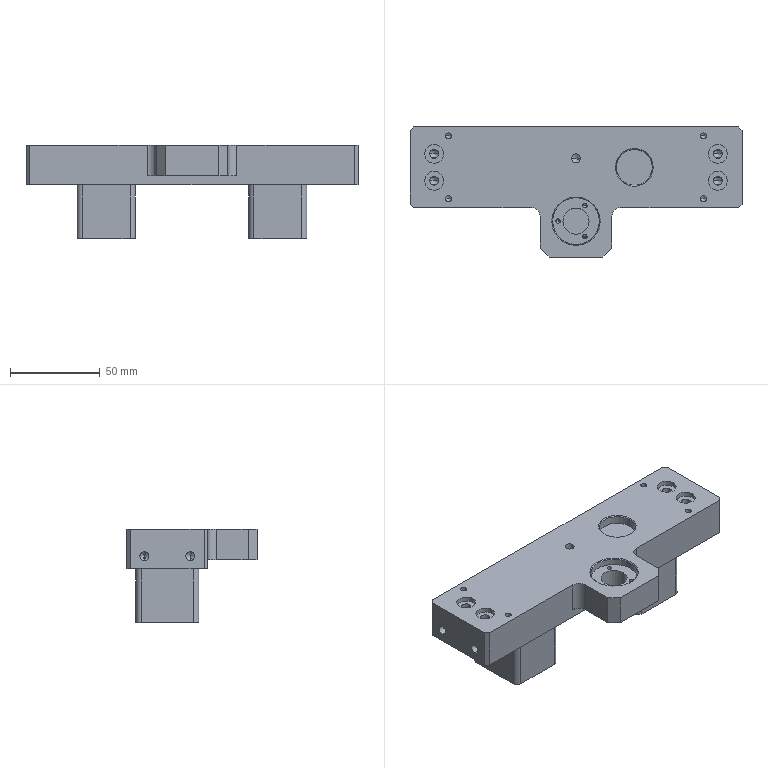Part | 1 solid | 334 faces | box 185 x 72.5 x 52 mm | volume 250671 mm3 | cylinder 128 | plane 95 | cone 56 | spline 55 | commonest cylinder face diameters 5 x58 4.2 x32 3.3 x8 6 x8 10.5 x8 2.5 x6